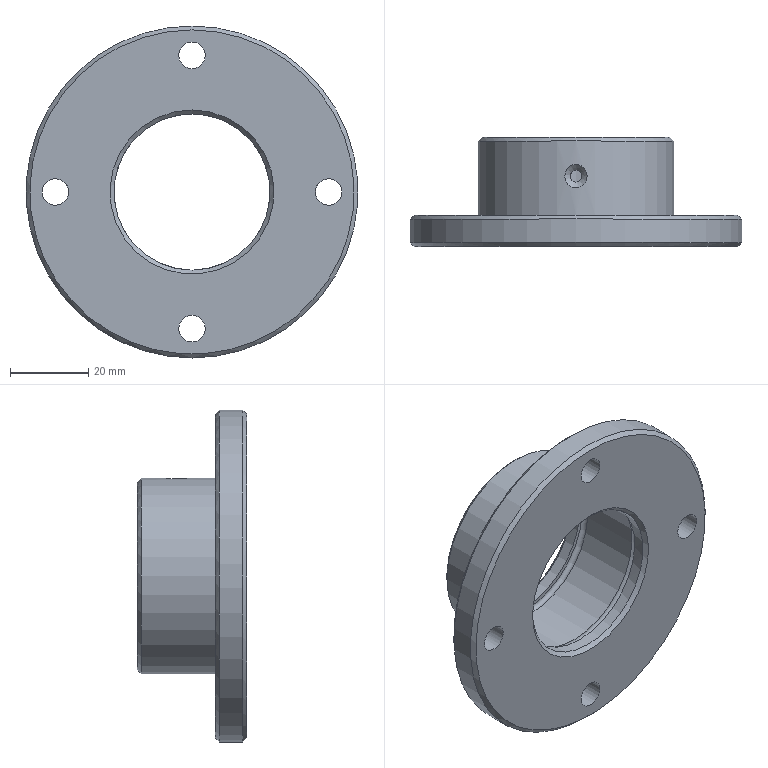Part | NX | features SYMBOLIC_THREAD 4, IDENTICAL INSTANCE OUTPUT 3, Instance Feature 3, DATUM_CSYS 2, HOLE PACKAGE 2, CHAMFER 1, CSUNK_HOLE 1, MASTER SNAPSHOT BODY 1, Pattern Feature 1, SIMPLE HOLE 1, SKETCH 1, SWP104 1 | 1 solid | 23 faces | box 85 x 28 x 85 mm | volume 44808 mm3 | cylinder 10 | cone 6 | plane 5 | torus 2 | commonest cylinder face diameters 6.8 x4 40 x2 3 x1 42 x1 50 x1 85 x1
STEP:
#1=CARTESIAN_POINT('',(38.4,0.,0.));
#2=VERTEX_POINT('',#1);
#3=CARTESIAN_POINT('',(35.,0.,0.));
#4=DIRECTION('',(0.,1.,0.));
#5=DIRECTION('',(1.,0.,0.));
#6=AXIS2_PLACEMENT_3D('',#3,#4,#5);
#7=CIRCLE('',#6,3.4);
#8=EDGE_CURVE('',#2,#2,#7,.T.);
#9=ORIENTED_EDGE('',*,*,#8,.T.);
#10=EDGE_LOOP('',(#9));
#11=FACE_BOUND('',#10,.T.);
#12=CARTESIAN_POINT('',(0.,0.,-38.4));
#13=VERTEX_POINT('',#12);
#14=CARTESIAN_POINT('',(0.,0.,-35.));
#15=DIRECTION('',(0.,1.,0.));
#16=DIRECTION('',(0.,0.,-1.));
#17=AXIS2_PLACEMENT_3D('',#14,#15,#16);
#18=CIRCLE('',#17,3.4);
#19=EDGE_CURVE('',#13,#13,#18,.T.);
#20=ORIENTED_EDGE('',*,*,#19,.T.);
#21=EDGE_LOOP('',(#20));
#22=FACE_BOUND('',#21,.T.);
#23=CARTESIAN_POINT('',(-38.4,0.,0.));
#24=VERTEX_POINT('',#23);
#25=CARTESIAN_POINT('',(-35.,0.,0.));
#26=DIRECTION('',(0.,1.,0.));
#27=DIRECTION('',(-1.,0.,0.));
#28=AXIS2_PLACEMENT_3D('',#25,#26,#27);
#29=CIRCLE('',#28,3.4);
#30=EDGE_CURVE('',#24,#24,#29,.T.);
#31=ORIENTED_EDGE('',*,*,#30,.T.);
#32=EDGE_LOOP('',(#31));
#33=FACE_BOUND('',#32,.T.);
#34=CARTESIAN_POINT('',(0.,0.,38.4));
#35=VERTEX_POINT('',#34);
#36=CARTESIAN_POINT('',(0.,0.,35.));
#37=DIRECTION('',(0.,1.,0.));
#38=DIRECTION('',(0.,0.,1.));
#39=AXIS2_PLACEMENT_3D('',#36,#37,#38);
#40=CIRCLE('',#39,3.4);
#41=EDGE_CURVE('',#35,#35,#40,.T.);
#42=ORIENTED_EDGE('',*,*,#41,.T.);
#43=EDGE_LOOP('',(#42));
#44=FACE_BOUND('',#43,.T.);
#45=CARTESIAN_POINT('',(0.,0.,21.));
#46=VERTEX_POINT('',#45);
#47=CARTESIAN_POINT('',(0.,0.,0.));
#48=DIRECTION('',(0.,1.,0.));
#49=DIRECTION('',(0.,0.,1.));
#50=AXIS2_PLACEMENT_3D('',#47,#48,#49);
#51=CIRCLE('',#50,21.);
#52=EDGE_CURVE('',#46,#46,#51,.T.);
#53=ORIENTED_EDGE('',*,*,#52,.T.);
#54=EDGE_LOOP('',(#53));
#55=FACE_BOUND('',#54,.T.);
#56=CARTESIAN_POINT('',(0.,0.,41.5));
#57=VERTEX_POINT('',#56);
#58=CARTESIAN_POINT('',(0.,0.,0.));
#59=DIRECTION('',(0.,1.,0.));
#60=DIRECTION('',(0.,0.,1.));
#61=AXIS2_PLACEMENT_3D('',#58,#59,#60);
#62=CIRCLE('',#61,41.5);
#63=EDGE_CURVE('',#57,#57,#62,.F.);
#64=ORIENTED_EDGE('',*,*,#63,.T.);
#65=EDGE_LOOP('',(#64));
#66=FACE_BOUND('',#65,.T.);
#67=CARTESIAN_POINT('',(0.,0.,42.5));
#68=DIRECTION('',(0.,1.,0.));
#69=DIRECTION('',(0.,0.,1.));
#70=AXIS2_PLACEMENT_3D('',#67,#68,#69);
#71=PLANE('',#70);
#72=ADVANCED_FACE('',(#11,#22,#33,#44,#55,#66),#71,.F.);
#73=CARTESIAN_POINT('',(0.,1.,20.));
#74=VERTEX_POINT('',#73);
#75=CARTESIAN_POINT('',(0.,1.,0.));
#76=DIRECTION('',(0.,1.,0.));
#77=DIRECTION('',(0.,0.,1.));
#78=AXIS2_PLACEMENT_3D('',#75,#76,#77);
#79=CIRCLE('',#78,20.);
#80=EDGE_CURVE('',#74,#74,#79,.F.);
#81=ORIENTED_EDGE('',*,*,#80,.T.);
#82=EDGE_LOOP('',(#81));
#83=FACE_BOUND('',#82,.T.);
#84=CARTESIAN_POINT('',(0.,4.,-20.));
#85=VERTEX_POINT('',#84);
#86=CARTESIAN_POINT('',(0.,4.,0.));
#87=DIRECTION('',(0.,-1.,0.));
#88=DIRECTION('',(0.,0.,-1.));
#89=AXIS2_PLACEMENT_3D('',#86,#87,#88);
#90=CIRCLE('',#89,20.);
#91=EDGE_CURVE('',#85,#85,#90,.T.);
#92=ORIENTED_EDGE('',*,*,#91,.F.);
#93=EDGE_LOOP('',(#92));
#94=FACE_BOUND('',#93,.T.);
#95=CARTESIAN_POINT('',(0.,0.,0.));
#96=DIRECTION('',(0.,-1.,0.));
#97=DIRECTION('',(0.,0.,-1.));
#98=AXIS2_PLACEMENT_3D('',#95,#96,#97);
#99=CYLINDRICAL_SURFACE('',#98,20.);
#100=ADVANCED_FACE('',(#83,#94),#99,.F.);
#101=CARTESIAN_POINT('',(0.,4.,-21.));
#102=VERTEX_POINT('',#101);
#103=CARTESIAN_POINT('',(0.,4.,0.));
#104=DIRECTION('',(0.,-1.,0.));
#105=DIRECTION('',(0.,0.,-1.));
#106=AXIS2_PLACEMENT_3D('',#103,#104,#105);
#107=CIRCLE('',#106,21.);
#108=EDGE_CURVE('',#102,#102,#107,.T.);
#109=ORIENTED_EDGE('',*,*,#108,.F.);
#110=EDGE_LOOP('',(#109));
#111=FACE_BOUND('',#110,.T.);
#112=ORIENTED_EDGE('',*,*,#91,.T.);
#113=EDGE_LOOP('',(#112));
#114=FACE_BOUND('',#113,.T.);
#115=CARTESIAN_POINT('',(0.,4.,20.));
#116=DIRECTION('',(0.,-1.,0.));
#117=DIRECTION('',(0.,0.,-1.));
#118=AXIS2_PLACEMENT_3D('',#115,#116,#117);
#119=PLANE('',#118);
#120=ADVANCED_FACE('',(#111,#114),#119,.F.);
#121=CARTESIAN_POINT('',(0.,6.,-21.));
#122=VERTEX_POINT('',#121);
#123=CARTESIAN_POINT('',(0.,6.,0.));
#124=DIRECTION('',(0.,-1.,0.));
#125=DIRECTION('',(0.,0.,-1.));
#126=AXIS2_PLACEMENT_3D('',#123,#124,#125);
#127=CIRCLE('',#126,21.);
#128=EDGE_CURVE('',#122,#122,#127,.T.);
#129=ORIENTED_EDGE('',*,*,#128,.F.);
#130=EDGE_LOOP('',(#129));
#131=FACE_BOUND('',#130,.T.);
#132=ORIENTED_EDGE('',*,*,#108,.T.);
#133=EDGE_LOOP('',(#132));
#134=FACE_BOUND('',#133,.T.);
#135=CARTESIAN_POINT('',(0.,5.,0.));
#136=DIRECTION('',(0.,-1.,0.));
#137=DIRECTION('',(0.,0.,-1.));
#138=AXIS2_PLACEMENT_3D('',#135,#136,#137);
#139=TOROIDAL_SURFACE('',#138,21.,1.);
#140=ADVANCED_FACE('',(#131,#134),#139,.F.);
#141=CARTESIAN_POINT('',(-1.5,18.,20.946));
#142=VERTEX_POINT('',#141);
#143=CARTESIAN_POINT('',(-1.174,19.177,20.973));
#144=CARTESIAN_POINT('',(-1.663,18.,20.933));
#145=CARTESIAN_POINT('',(-1.175,16.824,20.973));
#146=CARTESIAN_POINT('',(-0.001255,16.338,21.013));
#147=CARTESIAN_POINT('',(1.175,16.824,20.973));
#148=CARTESIAN_POINT('',(1.662,18.,20.933));
#149=CARTESIAN_POINT('',(1.177,19.174,20.973));
#150=CARTESIAN_POINT('',(0.001699,19.662,21.013));
#151=CARTESIAN_POINT('',(-1.174,19.177,20.973));
#152=CARTESIAN_POINT('',(-1.663,18.,20.933));
#153=CARTESIAN_POINT('',(-1.175,16.824,20.973));
#154=B_SPLINE_CURVE_WITH_KNOTS('',3,(#143,#144,#145,#146,#147,#148,#149,#150,#151,#152,#153),.UNSPECIFIED.,.T.,.F.,(1,1,1,1,1,1,1,1,1,1,1,1,1,1,1),(-0.003518,-0.002345,-0.001173,0.,0.001173,0.002345,0.003518,0.004691,0.005863,0.007036,0.008209,0.009381,0.01055,0.01173,0.0129),.UNSPECIFIED.);
#155=EDGE_CURVE('',#142,#142,#154,.T.);
#156=ORIENTED_EDGE('',*,*,#155,.T.);
#157=EDGE_LOOP('',(#156));
#158=FACE_BOUND('',#157,.T.);
#159=CARTESIAN_POINT('',(0.,22.,-21.));
#160=VERTEX_POINT('',#159);
#161=CARTESIAN_POINT('',(0.,22.,0.));
#162=DIRECTION('',(0.,-1.,0.));
#163=DIRECTION('',(0.,0.,-1.));
#164=AXIS2_PLACEMENT_3D('',#161,#162,#163);
#165=CIRCLE('',#164,21.);
#166=EDGE_CURVE('',#160,#160,#165,.T.);
#167=ORIENTED_EDGE('',*,*,#166,.F.);
#168=EDGE_LOOP('',(#167));
#169=FACE_BOUND('',#168,.T.);
#170=ORIENTED_EDGE('',*,*,#128,.T.);
#171=EDGE_LOOP('',(#170));
#172=FACE_BOUND('',#171,.T.);
#173=CARTESIAN_POINT('',(0.,0.,0.));
#174=DIRECTION('',(0.,-1.,0.));
#175=DIRECTION('',(0.,0.,-1.));
#176=AXIS2_PLACEMENT_3D('',#173,#174,#175);
#177=CYLINDRICAL_SURFACE('',#176,21.);
#178=ADVANCED_FACE('',(#158,#169,#172),#177,.F.);
#179=CARTESIAN_POINT('',(0.,24.,-21.));
#180=VERTEX_POINT('',#179);
#181=CARTESIAN_POINT('',(0.,24.,0.));
#182=DIRECTION('',(0.,-1.,0.));
#183=DIRECTION('',(0.,0.,-1.));
#184=AXIS2_PLACEMENT_3D('',#181,#182,#183);
#185=CIRCLE('',#184,21.);
#186=EDGE_CURVE('',#180,#180,#185,.T.);
#187=ORIENTED_EDGE('',*,*,#186,.F.);
#188=EDGE_LOOP('',(#187));
#189=FACE_BOUND('',#188,.T.);
#190=ORIENTED_EDGE('',*,*,#166,.T.);
#191=EDGE_LOOP('',(#190));
#192=FACE_BOUND('',#191,.T.);
#193=CARTESIAN_POINT('',(0.,23.,0.));
#194=DIRECTION('',(0.,-1.,0.));
#195=DIRECTION('',(0.,0.,-1.));
#196=AXIS2_PLACEMENT_3D('',#193,#194,#195);
#197=TOROIDAL_SURFACE('',#196,21.,1.);
#198=ADVANCED_FACE('',(#189,#192),#197,.F.);
#199=CARTESIAN_POINT('',(0.,24.,-20.));
#200=VERTEX_POINT('',#199);
#201=CARTESIAN_POINT('',(0.,24.,0.));
#202=DIRECTION('',(0.,-1.,0.));
#203=DIRECTION('',(0.,0.,-1.));
#204=AXIS2_PLACEMENT_3D('',#201,#202,#203);
#205=CIRCLE('',#204,20.);
#206=EDGE_CURVE('',#200,#200,#205,.T.);
#207=ORIENTED_EDGE('',*,*,#206,.F.);
#208=EDGE_LOOP('',(#207));
#209=FACE_BOUND('',#208,.T.);
#210=ORIENTED_EDGE('',*,*,#186,.T.);
#211=EDGE_LOOP('',(#210));
#212=FACE_BOUND('',#211,.T.);
#213=CARTESIAN_POINT('',(0.,24.,21.));
#214=DIRECTION('',(0.,1.,0.));
#215=DIRECTION('',(0.,0.,1.));
#216=AXIS2_PLACEMENT_3D('',#213,#214,#215);
#217=PLANE('',#216);
#218=ADVANCED_FACE('',(#209,#212),#217,.F.);
#219=CARTESIAN_POINT('',(0.,27.,-20.));
#220=VERTEX_POINT('',#219);
#221=CARTESIAN_POINT('',(0.,27.,0.));
#222=DIRECTION('',(0.,-1.,0.));
#223=DIRECTION('',(0.,0.,-1.));
#224=AXIS2_PLACEMENT_3D('',#221,#222,#223);
#225=CIRCLE('',#224,20.);
#226=EDGE_CURVE('',#220,#220,#225,.F.);
#227=ORIENTED_EDGE('',*,*,#226,.T.);
#228=EDGE_LOOP('',(#227));
#229=FACE_BOUND('',#228,.T.);
#230=ORIENTED_EDGE('',*,*,#206,.T.);
#231=EDGE_LOOP('',(#230));
#232=FACE_BOUND('',#231,.T.);
#233=CARTESIAN_POINT('',(0.,0.,0.));
#234=DIRECTION('',(0.,-1.,0.));
#235=DIRECTION('',(0.,0.,-1.));
#236=AXIS2_PLACEMENT_3D('',#233,#234,#235);
#237=CYLINDRICAL_SURFACE('',#236,20.);
#238=ADVANCED_FACE('',(#229,#232),#237,.F.);
#239=CARTESIAN_POINT('',(0.,28.,-24.));
#240=VERTEX_POINT('',#239);
#241=CARTESIAN_POINT('',(0.,28.,0.));
#242=DIRECTION('',(0.,-1.,0.));
#243=DIRECTION('',(0.,0.,-1.));
#244=AXIS2_PLACEMENT_3D('',#241,#242,#243);
#245=CIRCLE('',#244,24.);
#246=EDGE_CURVE('',#240,#240,#245,.F.);
#247=ORIENTED_EDGE('',*,*,#246,.T.);
#248=EDGE_LOOP('',(#247));
#249=FACE_BOUND('',#248,.T.);
#250=CARTESIAN_POINT('',(0.,28.,-21.));
#251=VERTEX_POINT('',#250);
#252=CARTESIAN_POINT('',(0.,28.,0.));
#253=DIRECTION('',(0.,-1.,0.));
#254=DIRECTION('',(0.,0.,-1.));
#255=AXIS2_PLACEMENT_3D('',#252,#253,#254);
#256=CIRCLE('',#255,21.);
#257=EDGE_CURVE('',#251,#251,#256,.T.);
#258=ORIENTED_EDGE('',*,*,#257,.T.);
#259=EDGE_LOOP('',(#258));
#260=FACE_BOUND('',#259,.T.);
#261=CARTESIAN_POINT('',(0.,28.,20.));
#262=DIRECTION('',(0.,-1.,0.));
#263=DIRECTION('',(0.,0.,-1.));
#264=AXIS2_PLACEMENT_3D('',#261,#262,#263);
#265=PLANE('',#264);
#266=ADVANCED_FACE('',(#249,#260),#265,.F.);
#267=CARTESIAN_POINT('',(0.,27.,-25.));
#268=VERTEX_POINT('',#267);
#269=CARTESIAN_POINT('',(0.,27.,0.));
#270=DIRECTION('',(0.,-1.,0.));
#271=DIRECTION('',(0.,0.,-1.));
#272=AXIS2_PLACEMENT_3D('',#269,#270,#271);
#273=CIRCLE('',#272,25.);
#274=EDGE_CURVE('',#268,#268,#273,.T.);
#275=ORIENTED_EDGE('',*,*,#274,.T.);
#276=EDGE_LOOP('',(#275));
#277=FACE_BOUND('',#276,.T.);
#278=CARTESIAN_POINT('',(-2.059,15.937,24.915));
#279=VERTEX_POINT('',#278);
#280=CARTESIAN_POINT('',(-0.03678,14.649,25.043));
#281=CARTESIAN_POINT('',(-2.299,15.732,24.912));
#282=CARTESIAN_POINT('',(-3.122,18.044,24.8));
#283=CARTESIAN_POINT('',(-2.243,20.327,24.918));
#284=CARTESIAN_POINT('',(0.03617,21.351,25.042));
#285=CARTESIAN_POINT('',(2.298,20.269,24.912));
#286=CARTESIAN_POINT('',(3.121,17.962,24.8));
#287=CARTESIAN_POINT('',(2.246,15.675,24.918));
#288=CARTESIAN_POINT('',(-0.03678,14.649,25.043));
#289=CARTESIAN_POINT('',(-2.299,15.732,24.912));
#290=CARTESIAN_POINT('',(-3.122,18.044,24.8));
#291=B_SPLINE_CURVE_WITH_KNOTS('',3,(#280,#281,#282,#283,#284,#285,#286,#287,#288,#289,#290),.UNSPECIFIED.,.T.,.F.,(1,1,1,1,1,1,1,1,1,1,1,1,1,1,1),(-0.006873,-0.004582,-0.002291,0.,0.002291,0.004582,0.006873,0.009164,0.01146,0.01375,0.01604,0.01833,0.02062,0.02291,0.0252),.UNSPECIFIED.);
#292=EDGE_CURVE('',#279,#279,#291,.T.);
#293=ORIENTED_EDGE('',*,*,#292,.T.);
#294=EDGE_LOOP('',(#293));
#295=FACE_BOUND('',#294,.T.);
#296=CARTESIAN_POINT('',(0.,8.,-25.));
#297=VERTEX_POINT('',#296);
#298=CARTESIAN_POINT('',(0.,8.,0.));
#299=DIRECTION('',(0.,-1.,0.));
#300=DIRECTION('',(0.,0.,-1.));
#301=AXIS2_PLACEMENT_3D('',#298,#299,#300);
#302=CIRCLE('',#301,25.);
#303=EDGE_CURVE('',#297,#297,#302,.T.);
#304=ORIENTED_EDGE('',*,*,#303,.F.);
#305=EDGE_LOOP('',(#304));
#306=FACE_BOUND('',#305,.T.);
#307=CARTESIAN_POINT('',(0.,0.,0.));
#308=DIRECTION('',(0.,-1.,0.));
#309=DIRECTION('',(0.,0.,-1.));
#310=AXIS2_PLACEMENT_3D('',#307,#308,#309);
#311=CYLINDRICAL_SURFACE('',#310,25.);
#312=ADVANCED_FACE('',(#277,#295,#306),#311,.T.);
#313=CARTESIAN_POINT('',(35.,8.,-3.4));
#314=VERTEX_POINT('',#313);
#315=CARTESIAN_POINT('',(35.,8.,0.));
#316=DIRECTION('',(0.,-1.,0.));
#317=DIRECTION('',(0.,0.,-1.));
#318=AXIS2_PLACEMENT_3D('',#315,#316,#317);
#319=CIRCLE('',#318,3.4);
#320=EDGE_CURVE('',#314,#314,#319,.T.);
#321=ORIENTED_EDGE('',*,*,#320,.T.);
#322=EDGE_LOOP('',(#321));
#323=FACE_BOUND('',#322,.T.);
#324=CARTESIAN_POINT('',(0.,8.,-38.4));
#325=VERTEX_POINT('',#324);
#326=CARTESIAN_POINT('',(0.,8.,-35.));
#327=DIRECTION('',(0.,-1.,0.));
#328=DIRECTION('',(0.,0.,-1.));
#329=AXIS2_PLACEMENT_3D('',#326,#327,#328);
#330=CIRCLE('',#329,3.4);
#331=EDGE_CURVE('',#325,#325,#330,.T.);
#332=ORIENTED_EDGE('',*,*,#331,.T.);
#333=EDGE_LOOP('',(#332));
#334=FACE_BOUND('',#333,.T.);
#335=CARTESIAN_POINT('',(-35.,8.,-3.4));
#336=VERTEX_POINT('',#335);
#337=CARTESIAN_POINT('',(-35.,8.,0.));
#338=DIRECTION('',(0.,-1.,0.));
#339=DIRECTION('',(0.,0.,-1.));
#340=AXIS2_PLACEMENT_3D('',#337,#338,#339);
#341=CIRCLE('',#340,3.4);
#342=EDGE_CURVE('',#336,#336,#341,.T.);
#343=ORIENTED_EDGE('',*,*,#342,.T.);
#344=EDGE_LOOP('',(#343));
#345=FACE_BOUND('',#344,.T.);
#346=CARTESIAN_POINT('',(0.,8.,31.6));
#347=VERTEX_POINT('',#346);
#348=CARTESIAN_POINT('',(0.,8.,35.));
#349=DIRECTION('',(0.,-1.,0.));
#350=DIRECTION('',(0.,0.,-1.));
#351=AXIS2_PLACEMENT_3D('',#348,#349,#350);
#352=CIRCLE('',#351,3.4);
#353=EDGE_CURVE('',#347,#347,#352,.T.);
#354=ORIENTED_EDGE('',*,*,#353,.T.);
#355=EDGE_LOOP('',(#354));
#356=FACE_BOUND('',#355,.T.);
#357=CARTESIAN_POINT('',(0.,8.,-41.5));
#358=VERTEX_POINT('',#357);
#359=CARTESIAN_POINT('',(0.,8.,0.));
#360=DIRECTION('',(0.,-1.,0.));
#361=DIRECTION('',(0.,0.,-1.));
#362=AXIS2_PLACEMENT_3D('',#359,#360,#361);
#363=CIRCLE('',#362,41.5);
#364=EDGE_CURVE('',#358,#358,#363,.F.);
#365=ORIENTED_EDGE('',*,*,#364,.T.);
#366=EDGE_LOOP('',(#365));
#367=FACE_BOUND('',#366,.T.);
#368=ORIENTED_EDGE('',*,*,#303,.T.);
#369=EDGE_LOOP('',(#368));
#370=FACE_BOUND('',#369,.T.);
#371=CARTESIAN_POINT('',(0.,8.,25.));
#372=DIRECTION('',(0.,-1.,0.));
#373=DIRECTION('',(0.,0.,-1.));
#374=AXIS2_PLACEMENT_3D('',#371,#372,#373);
#375=PLANE('',#374);
#376=ADVANCED_FACE('',(#323,#334,#345,#356,#367,#370),#375,.F.);
#377=CARTESIAN_POINT('',(0.,7.,-42.5));
#378=VERTEX_POINT('',#377);
#379=CARTESIAN_POINT('',(0.,7.,0.));
#380=DIRECTION('',(0.,-1.,0.));
#381=DIRECTION('',(0.,0.,-1.));
#382=AXIS2_PLACEMENT_3D('',#379,#380,#381);
#383=CIRCLE('',#382,42.5);
#384=EDGE_CURVE('',#378,#378,#383,.T.);
#385=ORIENTED_EDGE('',*,*,#384,.T.);
#386=EDGE_LOOP('',(#385));
#387=FACE_BOUND('',#386,.T.);
#388=CARTESIAN_POINT('',(0.,1.,42.5));
#389=VERTEX_POINT('',#388);
#390=CARTESIAN_POINT('',(0.,1.,0.));
#391=DIRECTION('',(0.,1.,0.));
#392=DIRECTION('',(0.,0.,1.));
#393=AXIS2_PLACEMENT_3D('',#390,#391,#392);
#394=CIRCLE('',#393,42.5);
#395=EDGE_CURVE('',#389,#389,#394,.T.);
#396=ORIENTED_EDGE('',*,*,#395,.T.);
#397=EDGE_LOOP('',(#396));
#398=FACE_BOUND('',#397,.T.);
#399=CARTESIAN_POINT('',(0.,0.,0.));
#400=DIRECTION('',(0.,-1.,0.));
#401=DIRECTION('',(0.,0.,-1.));
#402=AXIS2_PLACEMENT_3D('',#399,#400,#401);
#403=CYLINDRICAL_SURFACE('',#402,42.5);
#404=ADVANCED_FACE('',(#387,#398),#403,.T.);
#405=CARTESIAN_POINT('',(-1.5,18.,23.5));
#406=VERTEX_POINT('',#405);
#407=CARTESIAN_POINT('',(0.,18.,23.5));
#408=DIRECTION('',(0.,0.,-1.));
#409=DIRECTION('',(-1.,0.,0.));
#410=AXIS2_PLACEMENT_3D('',#407,#408,#409);
#411=CIRCLE('',#410,1.5);
#412=EDGE_CURVE('',#406,#406,#411,.F.);
#413=ORIENTED_EDGE('',*,*,#412,.F.);
#414=EDGE_LOOP('',(#413));
#415=FACE_BOUND('',#414,.T.);
#416=ORIENTED_EDGE('',*,*,#292,.F.);
#417=EDGE_LOOP('',(#416));
#418=FACE_BOUND('',#417,.T.);
#419=CARTESIAN_POINT('',(0.,18.,25.));
#420=DIRECTION('',(0.,0.,1.));
#421=DIRECTION('',(1.,0.,0.));
#422=AXIS2_PLACEMENT_3D('',#419,#420,#421);
#423=CONICAL_SURFACE('',#422,3.,0.7854);
#424=ADVANCED_FACE('',(#415,#418),#423,.F.);
#425=ORIENTED_EDGE('',*,*,#412,.T.);
#426=EDGE_LOOP('',(#425));
#427=FACE_BOUND('',#426,.T.);
#428=ORIENTED_EDGE('',*,*,#155,.F.);
#429=EDGE_LOOP('',(#428));
#430=FACE_BOUND('',#429,.T.);
#431=CARTESIAN_POINT('',(0.,18.,-495000.));
#432=DIRECTION('',(0.,0.,-1.));
#433=DIRECTION('',(-1.,0.,0.));
#434=AXIS2_PLACEMENT_3D('',#431,#432,#433);
#435=CYLINDRICAL_SURFACE('',#434,1.5);
#436=ADVANCED_FACE('',(#427,#430),#435,.F.);
#437=ORIENTED_EDGE('',*,*,#246,.F.);
#438=EDGE_LOOP('',(#437));
#439=FACE_BOUND('',#438,.T.);
#440=ORIENTED_EDGE('',*,*,#274,.F.);
#441=EDGE_LOOP('',(#440));
#442=FACE_BOUND('',#441,.T.);
#443=CARTESIAN_POINT('',(0.,27.,0.));
#444=DIRECTION('',(0.,-1.,0.));
#445=DIRECTION('',(0.,0.,-1.));
#446=AXIS2_PLACEMENT_3D('',#443,#444,#445);
#447=CONICAL_SURFACE('',#446,25.,0.7854);
#448=ADVANCED_FACE('',(#439,#442),#447,.T.);
#449=ORIENTED_EDGE('',*,*,#226,.F.);
#450=EDGE_LOOP('',(#449));
#451=FACE_BOUND('',#450,.T.);
#452=ORIENTED_EDGE('',*,*,#257,.F.);
#453=EDGE_LOOP('',(#452));
#454=FACE_BOUND('',#453,.T.);
#455=CARTESIAN_POINT('',(0.,28.,0.));
#456=DIRECTION('',(0.,1.,0.));
#457=DIRECTION('',(0.,0.,1.));
#458=AXIS2_PLACEMENT_3D('',#455,#456,#457);
#459=CONICAL_SURFACE('',#458,21.,0.7854);
#460=ADVANCED_FACE('',(#451,#454),#459,.F.);
#461=ORIENTED_EDGE('',*,*,#52,.F.);
#462=EDGE_LOOP('',(#461));
#463=FACE_BOUND('',#462,.T.);
#464=ORIENTED_EDGE('',*,*,#80,.F.);
#465=EDGE_LOOP('',(#464));
#466=FACE_BOUND('',#465,.T.);
#467=CARTESIAN_POINT('',(0.,1.,0.));
#468=DIRECTION('',(0.,-1.,0.));
#469=DIRECTION('',(0.,0.,-1.));
#470=AXIS2_PLACEMENT_3D('',#467,#468,#469);
#471=CONICAL_SURFACE('',#470,20.,0.7854);
#472=ADVANCED_FACE('',(#463,#466),#471,.F.);
#473=ORIENTED_EDGE('',*,*,#364,.F.);
#474=EDGE_LOOP('',(#473));
#475=FACE_BOUND('',#474,.T.);
#476=ORIENTED_EDGE('',*,*,#384,.F.);
#477=EDGE_LOOP('',(#476));
#478=FACE_BOUND('',#477,.T.);
#479=CARTESIAN_POINT('',(0.,7.,0.));
#480=DIRECTION('',(0.,-1.,0.));
#481=DIRECTION('',(0.,0.,-1.));
#482=AXIS2_PLACEMENT_3D('',#479,#480,#481);
#483=CONICAL_SURFACE('',#482,42.5,0.7854);
#484=ADVANCED_FACE('',(#475,#478),#483,.T.);
#485=ORIENTED_EDGE('',*,*,#395,.F.);
#486=EDGE_LOOP('',(#485));
#487=FACE_BOUND('',#486,.T.);
#488=ORIENTED_EDGE('',*,*,#63,.F.);
#489=EDGE_LOOP('',(#488));
#490=FACE_BOUND('',#489,.T.);
#491=CARTESIAN_POINT('',(0.,0.,0.));
#492=DIRECTION('',(0.,1.,0.));
#493=DIRECTION('',(0.,0.,1.));
#494=AXIS2_PLACEMENT_3D('',#491,#492,#493);
#495=CONICAL_SURFACE('',#494,41.5,0.7854);
#496=ADVANCED_FACE('',(#487,#490),#495,.T.);
#497=ORIENTED_EDGE('',*,*,#41,.F.);
#498=EDGE_LOOP('',(#497));
#499=FACE_BOUND('',#498,.T.);
#500=ORIENTED_EDGE('',*,*,#353,.F.);
#501=EDGE_LOOP('',(#500));
#502=FACE_BOUND('',#501,.T.);
#503=CARTESIAN_POINT('',(0.,0.,35.));
#504=DIRECTION('',(0.,1.,0.));
#505=DIRECTION('',(0.,0.,1.));
#506=AXIS2_PLACEMENT_3D('',#503,#504,#505);
#507=CYLINDRICAL_SURFACE('',#506,3.4);
#508=ADVANCED_FACE('',(#499,#502),#507,.F.);
#509=ORIENTED_EDGE('',*,*,#30,.F.);
#510=EDGE_LOOP('',(#509));
#511=FACE_BOUND('',#510,.T.);
#512=ORIENTED_EDGE('',*,*,#342,.F.);
#513=EDGE_LOOP('',(#512));
#514=FACE_BOUND('',#513,.T.);
#515=CARTESIAN_POINT('',(-35.,0.,0.));
#516=DIRECTION('',(0.,1.,0.));
#517=DIRECTION('',(-1.,0.,0.));
#518=AXIS2_PLACEMENT_3D('',#515,#516,#517);
#519=CYLINDRICAL_SURFACE('',#518,3.4);
#520=ADVANCED_FACE('',(#511,#514),#519,.F.);
#521=ORIENTED_EDGE('',*,*,#19,.F.);
#522=EDGE_LOOP('',(#521));
#523=FACE_BOUND('',#522,.T.);
#524=ORIENTED_EDGE('',*,*,#331,.F.);
#525=EDGE_LOOP('',(#524));
#526=FACE_BOUND('',#525,.T.);
#527=CARTESIAN_POINT('',(0.,0.,-35.));
#528=DIRECTION('',(0.,1.,0.));
#529=DIRECTION('',(0.,0.,-1.));
#530=AXIS2_PLACEMENT_3D('',#527,#528,#529);
#531=CYLINDRICAL_SURFACE('',#530,3.4);
#532=ADVANCED_FACE('',(#523,#526),#531,.F.);
#533=ORIENTED_EDGE('',*,*,#8,.F.);
#534=EDGE_LOOP('',(#533));
#535=FACE_BOUND('',#534,.T.);
#536=ORIENTED_EDGE('',*,*,#320,.F.);
#537=EDGE_LOOP('',(#536));
#538=FACE_BOUND('',#537,.T.);
#539=CARTESIAN_POINT('',(35.,0.,0.));
#540=DIRECTION('',(0.,1.,0.));
#541=DIRECTION('',(1.,0.,0.));
#542=AXIS2_PLACEMENT_3D('',#539,#540,#541);
#543=CYLINDRICAL_SURFACE('',#542,3.4);
#544=ADVANCED_FACE('',(#535,#538),#543,.F.);
#545=CLOSED_SHELL('',(#72,#100,#120,#140,#178,#198,#218,#238,#266,#312,#376,#404,#424,#436,#448,#460,#472,#484,#496,#508,#520,#532,#544));
#546=MANIFOLD_SOLID_BREP('',#545);
#547=(LENGTH_UNIT()NAMED_UNIT(*)SI_UNIT(.MILLI.,.METRE.));
#548=UNCERTAINTY_MEASURE_WITH_UNIT(LENGTH_MEASURE(0.0508),#547,'','');
#549=(NAMED_UNIT(*)PLANE_ANGLE_UNIT()SI_UNIT($,.RADIAN.));
#550=(NAMED_UNIT(*)SI_UNIT($,.STERADIAN.)SOLID_ANGLE_UNIT());
#551=(GEOMETRIC_REPRESENTATION_CONTEXT(3)GLOBAL_UNCERTAINTY_ASSIGNED_CONTEXT((#548))GLOBAL_UNIT_ASSIGNED_CONTEXT((#547,#549,#550))REPRESENTATION_CONTEXT('',''));
#552=ADVANCED_BREP_SHAPE_REPRESENTATION('',(#546),#551);